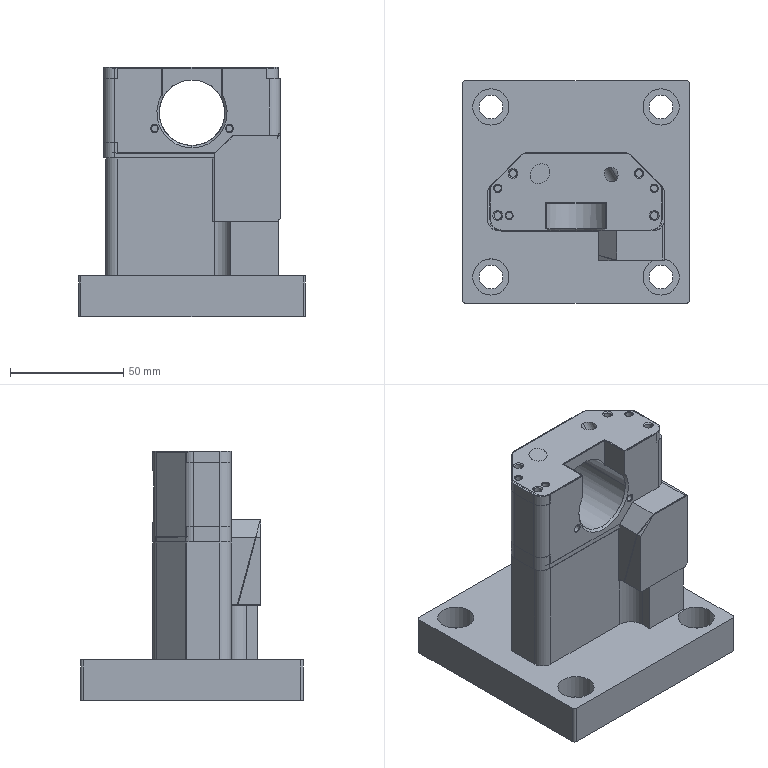NC program | NX | posted with a generic post | part box 100 x 98 x 110 mm
Lines 5823 to 6635 of 6635:
(3_AXIS_DEBURRING , TOOL : R1.75)
N11374 T07 M6
N11376 G54
N11378 G17 G0 G90 X41.123 Y0.273 B0. C0. S4500 M3
N11380 G43 Z67.959 H7
N11382 Z35.96
N11384 G94 G1 X41.109 Y0.272 Z35.792 F540.
N11386 X41.071 Y0.27 Z35.627
N11388 X41.011 Y0.267 Z35.466
N11390 X40.933 Y0.263 Z35.309
N11392 X40.736 Y0.251 Z35.017
N11394 X40.505 Y0.239 Z34.758
N11396 X40.415 Y0.21 Z34.668
N11398 X40.335 Y0.142 Z34.587
N11400 X40.264 Y0.042 Z34.517
N11402 X40.205 Y-0.082 Z34.457
N11404 X40.158 Y-0.222 Z34.41
N11406 X40.123 Y-0.371 Z34.375
N11408 X40.102 Y-0.519 Z34.353
N11410 X40.095 Y-0.66 Z34.346
N11412 X40.096 Y-1.682 F600.
N11414 Y-2.643
N11416 Y-3.603
N11418 Y-4.564
N11420 Y-5.525
N11422 Y-6.486
N11424 Y-7.446
N11426 Y-8.407
N11428 Y-9.368
N11430 Y-10.329
N11432 Y-11.289
N11434 Y-12.25
N11436 X40.104 Y-12.388 Z34.354
N11438 X40.126 Y-12.535 Z34.376
N11440 X40.161 Y-12.681 Z34.411
N11442 X40.209 Y-12.819 Z34.459
N11444 X40.269 Y-12.941 Z34.519
N11446 X40.339 Y-13.038 Z34.589
N11448 X40.42 Y-13.102 Z34.67
N11450 X40.508 Y-13.125 Z34.758
N11452 X40.74 Z35.017
N11454 X40.937 Z35.31
N11456 X41.015 Z35.466
N11458 X41.075 Z35.627
N11460 X41.114 Z35.793
N11462 X41.127 Z35.961
N11464 X41.164 Y-13.127 Z36.375
N11466 X41.206 Y-13.134 Z36.797
N11468 X41.254 Y-13.144 Z37.224
N11470 X41.306 Y-13.157 Z37.655
N11472 X41.36 Y-13.172 Z38.09
N11474 X41.416 Y-13.188 Z38.526
N11476 X41.473 Y-13.205 Z38.963
N11478 X41.528 Y-13.22 Z39.399
N11480 X41.582 Y-13.235 Z39.832
N11482 X41.632 Y-13.247 Z40.262
N11484 X41.678 Y-13.256 Z40.688
N11486 X41.719 Y-13.261 Z41.107
N11488 X41.753 Y-13.262 Z41.518
N11490 X41.78 Y-13.258 Z41.921
N11492 X41.797 Y-13.247 Z42.313
N11494 X41.805 Y-13.229 Z42.694
N11496 X41.801 Y-13.203 Z43.063
N11498 X41.784 Y-13.169 Z43.416
N11500 X41.754 Y-13.125 Z43.755
N11502 X41.704 Y-13.066 Z44.092
N11504 X41.629 Y-12.991 Z44.421
N11506 X41.531 Y-12.899 Z44.742
N11508 X41.411 Y-12.792 Z45.055
N11510 X41.268 Y-12.669 Z45.361
N11512 X41.104 Y-12.532 Z45.658
N11514 X40.919 Y-12.381 Z45.948
N11516 X40.714 Y-12.215 Z46.229
N11518 X40.49 Y-12.037 Z46.502
N11520 X40.247 Y-11.845 Z46.767
N11522 X39.986 Y-11.641 Z47.024
N11524 X39.707 Y-11.424 Z47.273
N11526 X39.412 Y-11.197 Z47.513
N11528 X39.101 Y-10.958 Z47.745
N11530 X38.774 Y-10.708 Z47.968
N11532 X38.433 Y-10.449 Z48.183
N11534 X38.077 Y-10.179 Z48.39
N11536 X37.708 Y-9.9 Z48.588
N11538 X37.327 Y-9.613 Z48.777
N11540 X36.933 Y-9.317 Z48.957
N11542 X36.528 Y-9.013 Z49.129
N11544 X36.112 Y-8.702 Z49.293
N11546 X35.686 Y-8.383 Z49.447
N11548 X35.251 Y-8.058 Z49.593
N11550 X34.807 Y-7.728 Z49.729
N11552 X34.355 Y-7.391 Z49.857
N11554 X33.895 Y-7.049 Z49.976
N11556 X33.429 Y-6.703 Z50.085
N11558 X32.956 Y-6.352 Z50.186
N11560 X32.478 Y-5.998 Z50.277
N11562 X31.996 Y-5.64 Z50.359
N11564 X31.509 Y-5.279 Z50.433
N11566 X31.019 Y-4.916 Z50.496
N11568 X30.526 Y-4.551 Z50.551
N11570 X30.031 Y-4.184 Z50.596
N11572 X29.535 Y-3.817 Z50.631
N11574 X29.038 Y-3.448 Z50.657
N11576 X28.541 Y-3.08 Z50.674
N11578 X28.044 Y-2.712 Z50.681
N11580 X27.549 Y-2.345 Z50.678
N11582 X27.055 Y-1.978 Z50.666
N11584 X26.564 Y-1.614 Z50.644
N11586 X26.076 Y-1.252 Z50.612
N11588 X25.592 Y-0.892 Z50.571
N11590 X25.113 Y-0.535 Z50.519
N11592 X24.639 Y-0.182 Z50.458
N11594 X24.171 Y0.167 Z50.387
N11596 X23.709 Y0.512 Z50.305
N11598 X23.255 Y0.851 Z50.214
N11600 X22.808 Y1.186 Z50.112
N11602 X22.37 Y1.515 Z50.001
N11604 X21.942 Y1.837 Z49.879
N11606 X21.523 Y2.153 Z49.747
N11608 X21.115 Y2.461 Z49.604
N11610 X20.717 Y2.762 Z49.452
N11612 X20.332 Y3.055 Z49.289
N11614 X19.959 Y3.339 Z49.115
N11616 X19.6 Y3.615 Z48.931
N11618 X19.254 Y3.881 Z48.736
N11620 X18.923 Y4.137 Z48.531
N11622 X18.607 Y4.382 Z48.315
N11624 X18.307 Y4.617 Z48.089
N11626 X18.024 Y4.841 Z47.851
N11628 X17.758 Y5.052 Z47.603
N11630 X17.509 Y5.252 Z47.345
N11632 X17.279 Y5.439 Z47.075
N11634 X17.069 Y5.613 Z46.794
N11636 X16.878 Y5.773 Z46.503
N11638 X16.708 Y5.919 Z46.2
N11640 X16.558 Y6.051 Z45.886
N11642 X16.431 Y6.168 Z45.561
N11644 X16.326 Y6.269 Z45.225
N11646 X16.245 Y6.355 Z44.878
N11648 X16.187 Y6.424 Z44.52
N11650 X16.154 Y6.476 Z44.15
N11652 X16.146 Y6.512 Z43.769
N11654 X16.149 Y6.521 Z43.623
N11656 X16.154 Y6.528 Z43.474
N11658 X16.162 Y6.534 Z43.323
N11660 X16.171 Y6.539 Z43.17
N11662 X16.182 Y6.543 Z43.016
N11664 X16.195 Y6.545 Z42.859
N11666 X16.209 Y6.547 Z42.701
N11668 X16.224 Y6.548 Z42.541
N11670 X16.24 Z42.381
N11672 X16.256 Z42.219
N11674 X16.274 Z42.058
N11676 X16.291 Y6.547 Z41.895
N11678 X16.309 Y6.546 Z41.733
N11680 X16.326 Y6.545 Z41.57
N11682 X16.344 Z41.408
N11684 X16.361 Y6.544 Z41.247
N11686 X16.377 Z41.086
N11688 X16.392 Y6.545 Z40.926
N11690 X16.406 Y6.547 Z40.768
N11692 X16.421 Y6.548 Z40.602 F540.
N11694 X16.462 Y6.554 Z40.439
N11696 X16.525 Y6.562 Z40.281
N11698 X16.607 Y6.573 Z40.129
N11700 X16.706 Y6.586 Z39.985
N11702 X16.815 Y6.601 Z39.848
N11704 X17.056 Y6.633 Z39.605
N11706 X17.147 Y6.669 Z39.523
N11708 X17.225 Y6.744 Z39.453
N11710 X17.289 Y6.851 Z39.393
N11712 X17.34 Y6.98 Z39.345
N11714 X17.377 Y7.124 Z39.309
N11716 X17.401 Y7.274 Z39.285
N11718 X17.41 Y7.422 Z39.273
N11720 X17.404 Y7.56 Z39.275
N11722 X17.395 Y7.661 Z39.282 F600.
N11724 X17.384 Y7.766 Z39.288
N11726 X17.35 Y7.904 Z39.303
N11728 X17.316 Y8.043 Z39.317
N11730 X17.281 Y8.181 Z39.332
N11732 X17.247 Y8.32 Z39.346
N11734 X17.19 Y8.444 Z39.359
N11736 X17.133 Y8.567 Z39.372
N11738 X17.076 Y8.691 Z39.385
N11740 X16.985 Y8.824 Z39.4
N11742 X16.894 Y8.957 Z39.414
N11744 X16.804 Y9.09 Z39.429
N11746 X16.674 Y9.213 Z39.442
N11748 X16.545 Y9.336 Z39.454
N11750 X16.415 Y9.459 Z39.467
N11752 X16.279 Y9.556 Z39.482
N11754 X16.142 Y9.654 Z39.498
N11756 X16.002 Y9.715 Z39.506
N11758 X15.861 Y9.777 Z39.515
N11760 X15.721 Y9.838 Z39.523
N11762 X15.555 Y9.867 Z39.529
N11764 X15.388 Y9.895 Z39.535
N11766 X15.222 Y9.924 Z39.541
N11768 X15.062 Y9.923 Z39.548
N11770 X14.902 Y9.922 Z39.556
N11772 X14.753 Y9.893 Z39.563
N11774 X14.605 Y9.864 Z39.571
N11776 X14.456 Y9.835 Z39.578
N11778 X14.323 Y9.767 Z39.581
N11780 X14.19 Y9.699 Z39.584
N11782 X14.057 Y9.63 Z39.586
N11784 X13.942 Y9.513 Z39.582
N11786 X13.827 Y9.395 Z39.577
N11788 X13.713 Y9.277 Z39.572
N11790 X13.641 Y9.154 Z39.567
N11792 X13.569 Y9.031 Z39.561
N11794 X13.497 Y8.907 Z39.556
N11796 X13.448 Y8.755 Z39.545
N11798 X13.399 Y8.602 Z39.535
N11800 X13.375 Y8.425 Z39.525
N11802 X13.35 Y8.249 Z39.516
N11804 X13.326 Y8.072 Z39.507
N11806 X13.337 Y7.925 Z39.498
N11808 X13.348 Y7.777 Z39.489
N11810 X13.359 Y7.63 Z39.481
N11812 X13.397 Y7.461 Z39.472
N11814 X13.434 Y7.293 Z39.463
N11816 X13.518 Y7.111 Z39.447
N11818 X13.602 Y6.93 Z39.432
N11820 X13.686 Y6.748 Z39.416
N11822 X13.778 Y6.644 Z39.391
N11824 X13.87 Y6.539 Z39.366
N11826 X13.962 Y6.435 Z39.341
N11828 X14.066 Y6.32 Z39.335
N11830 X14.171 Y6.206 Z39.328
N11832 X14.276 Y6.091 Z39.322
N11834 X14.412 Y5.994 Z39.312
N11836 X14.549 Y5.897 Z39.302
N11838 X14.685 Y5.8 Z39.292
N11840 X14.784 Y5.773 Z39.264
N11842 X14.883 Y5.745 Z39.236
N11844 X14.982 Y5.717 Z39.209
N11846 X15.076 Y5.688 Z39.204
N11848 X15.17 Y5.659 Z39.2
N11850 X15.265 Y5.63 Z39.195
N11852 X15.359 Y5.601 Z39.191
N11854 X15.464 Y5.597 Z39.178
N11856 X15.568 Y5.594 Z39.166
N11858 X15.673 Y5.59 Z39.153
N11860 X15.777 Y5.587 Z39.141
N11862 X15.86 Y5.601 Z39.13
N11864 X15.943 Y5.615 Z39.119
N11866 X16.027 Y5.629 Z39.108
N11868 X16.111 Y5.646 Z39.117
N11870 X16.196 Y5.663 Z39.126
N11872 X16.281 Y5.68 Z39.135
N11874 X16.366 Y5.697 Z39.144
N11876 X16.436 Y5.748 Z39.129
N11878 X16.506 Y5.798 Z39.113
N11880 X16.575 Y5.849 Z39.098
N11882 X16.645 Y5.899 Z39.082
N11884 X16.717 Y5.955 Z39.095
N11886 X16.788 Y6.01 Z39.108
N11888 X16.86 Y6.065 Z39.121
N11890 X16.931 Y6.121 Z39.133
N11892 X16.983 Y6.187 Z39.142
N11894 X17.034 Y6.254 Z39.15
N11896 X17.085 Y6.32 Z39.158
N11898 X17.137 Y6.386 Z39.167
N11900 X17.169 Y6.466 Z39.164
N11902 X17.201 Y6.546 Z39.161
N11904 X17.233 Y6.626 Z39.158
N11906 X17.264 Y6.734 Z39.167
N11908 X17.294 Y6.843 Z39.176
N11910 X17.324 Y6.951 Z39.186
N11912 X17.354 Y7.06 Z39.195
N11914 X17.374 Y7.19 Z39.219
N11916 X17.395 Y7.321 Z39.243
N11918 X17.415 Y7.451 Z39.268
N11920 X17.405 Y7.556 Z39.275
N11922 X17.404 Y7.56
N11924 X17.383 Y7.697 Z39.291
N11926 X17.346 Y7.84 Z39.321
N11928 X17.294 Y7.98 Z39.363
N11930 X17.231 Y8.11 Z39.417
N11932 X17.156 Y8.222 Z39.481
N11934 X17.073 Y8.309 Z39.553
N11936 X16.982 Y8.361 Z39.633
N11938 X16.886 Y8.371 Z39.718
N11940 X16.645 Y8.339 Z39.961
N11942 X16.535 Y8.324 Z40.098
N11944 X16.437 Y8.311 Z40.243
N11946 X16.354 Y8.3 Z40.395
N11948 X16.291 Y8.292 Z40.553
N11950 X16.25 Y8.286 Z40.715
N11952 X16.236 Y8.284 Z40.881
N11954 G0 Z45.881
N11956 G1 X16.232 Z46.073
N11958 X16.221 Z46.263
N11960 X16.202 Z46.451
N11962 X16.176 Y8.283 Z46.636
N11964 X16.142 Z46.818
N11966 X16.102 Y8.282 Z46.999
N11968 X16.054 Y8.281 Z47.176
N11970 X16. Y8.28 Z47.352
N11972 X15.939 Y8.278 Z47.525
N11974 X15.871 Y8.277 Z47.695
N11976 X15.796 Y8.276 Z47.863
N11978 X15.715 Y8.274 Z48.029
N11980 X15.627 Y8.272 Z48.192
N11982 X15.533 Y8.27 Z48.353
N11984 X15.433 Y8.268 Z48.511
N11986 X15.327 Y8.266 Z48.667
N11988 X15.214 Y8.264 Z48.82
N11990 X15.096 Y8.261 Z48.971
N11992 X14.972 Y8.259 Z49.12
N11994 X14.842 Y8.256 Z49.266
N11996 X14.707 Y8.254 Z49.409
N11998 X14.566 Y8.251 Z49.55
N12000 X14.42 Y8.248 Z49.689
N12002 X14.268 Y8.245 Z49.825
N12004 X14.111 Y8.242 Z49.959
N12006 X13.949 Y8.238 Z50.09
N12008 X13.782 Y8.235 Z50.219
N12010 X13.61 Y8.231 Z50.346
N12012 X13.433 Y8.228 Z50.47
N12014 X13.251 Y8.224 Z50.591
N12016 X13.065 Y8.22 Z50.71
N12018 X12.874 Y8.217 Z50.826
N12020 X12.679 Y8.213 Z50.941
N12022 X12.48 Y8.209 Z51.052
N12024 X12.276 Y8.204 Z51.161
N12026 X12.068 Y8.2 Z51.268
N12028 X11.856 Y8.196 Z51.372
N12030 X11.641 Y8.192 Z51.474
N12032 X11.421 Y8.187 Z51.573
N12034 X11.198 Y8.183 Z51.669
N12036 X10.971 Y8.178 Z51.764
N12038 X10.741 Y8.173 Z51.855
N12040 X10.507 Y8.169 Z51.944
N12042 X10.27 Y8.164 Z52.031
N12044 X10.029 Y8.159 Z52.115
N12046 X9.786 Y8.154 Z52.197
N12048 X9.539 Y8.149 Z52.276
N12050 X9.29 Y8.144 Z52.353
N12052 X9.038 Y8.139 Z52.427
N12054 X8.783 Y8.134 Z52.499
N12056 X8.525 Y8.129 Z52.568
N12058 X8.265 Y8.123 Z52.635
N12060 X8.003 Y8.118 Z52.699
N12062 X7.738 Y8.113 Z52.761
N12064 X7.471 Y8.107 Z52.82
N12066 X7.202 Y8.102 Z52.877
N12068 X6.931 Y8.096 Z52.931
N12070 X6.658 Y8.091 Z52.983
N12072 X6.383 Y8.085 Z53.032
N12074 X6.106 Y8.08 Z53.078
N12076 X5.828 Y8.074 Z53.122
N12078 X5.549 Y8.068 Z53.164
N12080 X5.268 Y8.063 Z53.203
N12082 X4.985 Y8.057 Z53.24
N12084 X4.702 Y8.051 Z53.274
N12086 X4.417 Y8.046 Z53.305
N12088 X4.131 Y8.04 Z53.334
N12090 X3.845 Y8.034 Z53.361
N12092 X3.557 Y8.028 Z53.384
N12094 X3.269 Y8.022 Z53.406
N12096 X2.981 Y8.017 Z53.425
N12098 X2.691 Y8.011 Z53.441
N12100 X2.402 Y8.005 Z53.455
N12102 X2.112 Y7.999 Z53.466
N12104 X1.822 Y7.993 Z53.474
N12106 X1.532 Y7.987 Z53.481
N12108 X1.241 Y7.981 Z53.484
N12110 X0.951 Y7.976 Z53.485
N12112 X0.661 Y7.97 Z53.484
N12114 X0.372 Y7.964 Z53.479
N12116 X0.083 Y7.958 Z53.473
N12118 X-0.206 Y7.952 Z53.464
N12120 X-0.494 Y7.946 Z53.452
N12122 X-0.782 Y7.94 Z53.438
N12124 X-1.068 Y7.935 Z53.421
N12126 X-1.354 Y7.929 Z53.401
N12128 X-1.639 Y7.923 Z53.379
N12130 X-1.922 Y7.917 Z53.355
N12132 X-2.204 Y7.912 Z53.328
N12134 X-2.486 Y7.906 Z53.298
N12136 X-2.765 Y7.9 Z53.266
N12138 X-3.043 Y7.895 Z53.231
N12140 X-3.32 Y7.889 Z53.193
N12142 X-3.595 Y7.884 Z53.153
N12144 X-3.868 Y7.878 Z53.111
N12146 X-4.139 Y7.873 Z53.066
N12148 X-4.408 Y7.867 Z53.018
N12150 X-4.675 Y7.862 Z52.968
N12152 X-4.94 Y7.856 Z52.915
N12154 X-5.202 Y7.851 Z52.859
N12156 X-5.462 Y7.846 Z52.801
N12158 X-5.72 Y7.841 Z52.741
N12160 X-5.975 Y7.836 Z52.677
N12162 X-6.227 Y7.83 Z52.612
N12164 X-6.476 Y7.825 Z52.543
N12166 X-6.723 Y7.82 Z52.472
N12168 X-6.966 Y7.815 Z52.398
N12170 X-7.207 Y7.811 Z52.322
N12172 X-7.444 Y7.806 Z52.243
N12174 X-7.677 Y7.801 Z52.162
N12176 X-7.908 Y7.796 Z52.078
N12178 X-8.135 Y7.792 Z51.991
N12180 X-8.358 Y7.787 Z51.902
N12182 X-8.578 Y7.783 Z51.81
N12184 X-8.793 Y7.779 Z51.716
N12186 X-9.005 Y7.774 Z51.619
N12188 X-9.213 Y7.77 Z51.519
N12190 X-9.417 Y7.766 Z51.417
N12192 X-9.616 Y7.762 Z51.312
N12194 X-9.811 Y7.758 Z51.204
N12196 X-10.002 Y7.754 Z51.094
N12198 X-10.188 Y7.75 Z50.981
N12200 X-10.37 Y7.747 Z50.866
N12202 X-10.547 Y7.743 Z50.748
N12204 X-10.719 Y7.74 Z50.627
N12206 X-10.886 Y7.736 Z50.504
N12208 X-11.048 Y7.733 Z50.378
N12210 X-11.205 Y7.73 Z50.25
N12212 X-11.356 Y7.727 Z50.119
N12214 X-11.503 Y7.724 Z49.985
N12216 X-11.644 Y7.721 Z49.848
N12218 X-11.779 Y7.718 Z49.709
N12220 X-11.909 Y7.716 Z49.567
N12222 X-12.033 Y7.713 Z49.423
N12224 X-12.151 Y7.711 Z49.276
N12226 X-12.264 Y7.708 Z49.126
N12228 X-12.37 Y7.706 Z48.974
N12230 X-12.47 Y7.704 Z48.819
N12232 X-12.564 Y7.702 Z48.662
N12234 X-12.652 Y7.701 Z48.501
N12236 X-12.733 Y7.699 Z48.338
N12238 X-12.808 Y7.697 Z48.173
N12240 X-12.876 Y7.696 Z48.005
N12242 X-12.937 Y7.695 Z47.834
N12244 X-12.991 Y7.694 Z47.66
N12246 X-13.039 Y7.693 Z47.484
N12248 X-13.079 Y7.692 Z47.305
N12250 X-13.113 Y7.691 Z47.124
N12252 X-13.139 Z46.939
N12254 X-13.158 Y7.69 Z46.753
N12256 X-13.169 Z46.563
N12258 X-13.173 Z46.371
N12260 G0 Z41.37
N12262 G1 X-13.163 Z41.195 F540.
N12264 X-13.135 Y7.689 Z41.022
N12266 X-13.034 Y7.688 Z40.681
N12268 X-12.886 Y7.685 Z40.354
N12270 X-12.709 Y7.682 Z40.045
N12272 X-12.642 Y7.705 Z39.939
N12274 X-12.581 Y7.768 Z39.844
N12276 X-12.526 Y7.864 Z39.761
N12278 X-12.478 Y7.985 Z39.692
N12280 X-12.439 Y8.123 Z39.636
N12282 X-12.409 Y8.269 Z39.595
N12284 X-12.39 Y8.414 Z39.571
N12286 X-12.381 Y8.552 Z39.564
N12288 X-12.379 Y8.626 Z39.565 F600.
N12290 X-12.375 Y8.839 Z39.568
N12292 X-12.377 Y9.048 Z39.582
N12294 X-12.378 Y9.257 Z39.596
N12296 X-12.431 Y9.451 Z39.594
N12298 X-12.483 Y9.644 Z39.592
N12300 X-12.556 Y9.863 Z39.599
N12302 X-12.63 Y10.081 Z39.607
N12304 X-12.692 Y10.227 Z39.617
N12306 X-12.754 Y10.373 Z39.626
N12308 X-12.877 Y10.516 Z39.62
N12310 X-12.999 Y10.66 Z39.613
N12312 X-13.184 Y10.849 Z39.619
N12314 X-13.368 Y11.038 Z39.624
N12316 X-13.621 Y11.186 Z39.622
N12318 X-13.874 Y11.334 Z39.619
N12320 X-14.054 Y11.392 Z39.614
N12322 X-14.235 Y11.45 Z39.608
N12324 X-14.481 Y11.526 Z39.614
N12326 X-14.747 Y11.538 Z39.603
N12328 X-15.013 Y11.55 Z39.591
N12330 X-15.215 Y11.543 Z39.59
N12332 X-15.417 Y11.537 Z39.589
N12334 X-15.622 Y11.482 Z39.575
N12336 X-15.826 Y11.427 Z39.56
N12338 X-16.033 Y11.364 Z39.555
N12340 X-16.239 Y11.302 Z39.55
N12342 X-16.433 Y11.2 Z39.534
N12344 X-16.626 Y11.098 Z39.517
N12346 X-16.868 Y10.957 Z39.509
N12348 X-17.11 Y10.817 Z39.502
N12350 X-17.24 Y10.698 Z39.482
N12352 X-17.369 Y10.579 Z39.462
N12354 X-17.533 Y10.409 Z39.439
N12356 X-17.698 Y10.24 Z39.416
N12358 X-17.861 Y10.076
N12360 X-18.024 Y9.913
N12362 X-18.139 Y9.73 Z39.39
N12364 X-18.254 Y9.548 Z39.364
N12366 X-18.432 Y9.207 Z39.333
N12368 X-18.61 Y8.865 Z39.301
N12370 X-18.668 Y8.678 Z39.277
N12372 X-18.727 Y8.49 Z39.253
N12374 X-18.785 Y8.302 Z39.229
N12376 X-18.835 Y8.069 Z39.218
N12378 X-18.886 Y7.837 Z39.207
N12380 X-18.936 Y7.604 Z39.196
N12382 X-18.949 Y7.483 Z39.197
N12384 X-18.963 Y7.362 Z39.198
N12386 X-18.976 Y7.241 Z39.199
N12388 X-18.961 Y7.128 Z39.178
N12390 X-18.946 Y7.016 Z39.157
N12392 X-18.931 Y6.903 Z39.136
N12394 X-18.91 Y6.707 Z39.139
N12396 X-18.889 Y6.511 Z39.141
N12398 X-18.846 Y6.408 Z39.115
N12400 X-18.802 Y6.305 Z39.088
N12402 X-18.759 Y6.202 Z39.062
N12404 X-18.718 Y6.082 Z39.073
N12406 X-18.678 Y5.963 Z39.084
N12408 X-18.637 Y5.843 Z39.095
N12410 X-18.582 Y5.779 Z39.068
N12412 X-18.527 Y5.715 Z39.041
N12414 X-18.471 Y5.652 Z39.014
N12416 X-18.422 Y5.567 Z39.033
N12418 X-18.373 Y5.482 Z39.053
N12420 X-18.324 Y5.397 Z39.072
N12422 X-18.247 Y5.33 Z39.065
N12424 X-18.169 Y5.263 Z39.057
N12426 X-18.092 Y5.196 Z39.05
N12428 X-18.015 Y5.129 Z39.043
N12430 X-17.916 Y5.075 Z39.033
N12432 X-17.817 Y5.022 Z39.023
N12434 X-17.718 Y4.968 Z39.013
N12436 X-17.619 Y4.914 Z39.003
N12438 X-17.532 Y4.863 Z39.032
N12440 X-17.446 Y4.812 Z39.06
N12442 X-17.36 Y4.761 Z39.088
N12444 X-17.259 Y4.747 Z39.069
N12446 X-17.158 Y4.733 Z39.049
N12448 X-17.013 Y4.71 Z39.058
N12450 X-16.868 Y4.687 Z39.067
N12452 X-16.723 Y4.664 Z39.076
N12454 X-16.609 Y4.649 Z39.101
N12456 X-16.496 Y4.635 Z39.127
N12458 X-16.383 Y4.621 Z39.153
N12460 X-16.202 Y4.651 Z39.147
N12462 X-16.022 Y4.682 Z39.142
N12464 X-15.893 Y4.698 Z39.165
N12466 X-15.764 Y4.714 Z39.189
N12468 X-15.635 Y4.73 Z39.213
N12470 X-15.454 Y4.806 Z39.206
N12472 X-15.273 Y4.882 Z39.2
N12474 X-15.032 Y4.992 Z39.221
N12476 X-14.791 Y5.102 Z39.242
N12478 X-14.653 Y5.185 Z39.251
N12480 X-14.516 Y5.269 Z39.26
N12482 X-14.33 Y5.399 Z39.279
N12484 X-14.143 Y5.53 Z39.297
N12486 X-13.959 Y5.666 Z39.333
N12488 X-13.774 Y5.802 Z39.368
N12490 X-13.626 Y5.957 Z39.381
N12492 X-13.478 Y6.113 Z39.395
N12494 X-13.258 Y6.433 Z39.41
N12496 X-13.037 Y6.754 Z39.425
N12498 X-12.933 Y6.934 Z39.444
N12500 X-12.83 Y7.114 Z39.463
N12502 X-12.727 Y7.294 Z39.482
N12504 X-12.603 Y7.651 Z39.505
N12506 X-12.479 Y8.009 Z39.528
N12508 X-12.431 Y8.211 Z39.545
N12510 X-12.384 Y8.413 Z39.562
N12512 X-12.381 Y8.552 Z39.564
N12514 X-12.384 Y8.691 Z39.575
N12516 X-12.397 Y8.838 Z39.603
N12518 X-12.42 Y8.984 Z39.648
N12520 X-12.453 Y9.123 Z39.708
N12522 X-12.495 Y9.245 Z39.781
N12524 X-12.546 Y9.343 Z39.867
N12526 X-12.605 Y9.408 Z39.964
N12528 X-12.671 Y9.432 Z40.072
N12530 X-12.848 Y9.435 Z40.381
N12532 X-12.996 Y9.437 Z40.708
N12534 X-13.097 Y9.439 Z41.048
N12536 X-13.125 Z41.222
N12538 X-13.135 Z41.397
N12540 G0 Z46.397
N12542 G1 X-13.138 Y9.436 Z46.635
N12544 X-13.149 Y9.428 Z46.867
N12546 X-13.167 Y9.413 Z47.095
N12548 X-13.192 Y9.393 Z47.318
N12550 X-13.224 Y9.368 Z47.537
N12552 X-13.262 Y9.337 Z47.752
N12554 X-13.307 Y9.3 Z47.962
N12556 X-13.359 Y9.258 Z48.167
N12558 X-13.418 Y9.211 Z48.368
N12560 X-13.482 Y9.159 Z48.565
N12562 X-13.553 Y9.102 Z48.757
N12564 X-13.631 Y9.04 Z48.945
N12566 X-13.714 Y8.972 Z49.129
N12568 X-13.803 Y8.9 Z49.309
N12570 X-13.899 Y8.824 Z49.484
N12572 X-14. Y8.742 Z49.654
N12574 X-14.107 Y8.656 Z49.821
N12576 X-14.219 Y8.565 Z49.983
N12578 X-14.338 Y8.47 Z50.141
N12580 X-14.461 Y8.37 Z50.295
N12582 X-14.59 Y8.266 Z50.445
N12584 X-14.724 Y8.158 Z50.59
N12586 X-14.864 Y8.046 Z50.732
N12588 X-15.008 Y7.929 Z50.869
N12590 X-15.157 Y7.809 Z51.002
N12592 X-15.312 Y7.685 Z51.131
N12594 X-15.471 Y7.556 Z51.256
N12596 X-15.634 Y7.424 Z51.377
N12598 X-15.803 Y7.289 Z51.494
N12600 X-15.976 Y7.149 Z51.606
N12602 X-16.153 Y7.007 Z51.715
N12604 X-16.334 Y6.86 Z51.82
N12606 X-16.52 Y6.71 Z51.921
N12608 X-16.71 Y6.557 Z52.018
N12610 X-16.904 Y6.401 Z52.111
N12612 X-17.102 Y6.242 Z52.2
N12614 X-17.303 Y6.079 Z52.285
N12616 X-17.509 Y5.914 Z52.366
N12618 X-17.718 Y5.745 Z52.444
N12620 X-17.93 Y5.574 Z52.517
N12622 X-18.146 Y5.4 Z52.587
N12624 X-18.365 Y5.223 Z52.653
N12626 X-18.588 Y5.044 Z52.715
N12628 X-18.814 Y4.862 Z52.774
N12630 X-19.042 Y4.677 Z52.829
N12632 X-19.274 Y4.49 Z52.88
N12634 X-19.509 Y4.301 Z52.927
N12636 X-19.746 Y4.11 Z52.97
N12638 X-19.986 Y3.916 Z53.01
N12640 X-20.229 Y3.721 Z53.047
N12642 X-20.474 Y3.523 Z53.079
N12644 X-20.722 Y3.324 Z53.108
N12646 X-20.971 Y3.122 Z53.134
N12648 X-21.223 Y2.919 Z53.156
N12650 X-21.478 Y2.714 Z53.174
N12652 X-21.734 Y2.508 Z53.189
N12654 X-21.992 Y2.3 Z53.2
N12656 X-22.252 Y2.09 Z53.208
N12658 X-22.513 Y1.88 Z53.212
N12660 X-22.776 Y1.667 Z53.213
N12662 X-23.041 Y1.454 Z53.21
N12664 X-23.307 Y1.239 Z53.204
N12666 X-23.575 Y1.024 Z53.195
N12668 X-23.844 Y0.807 Z53.182
N12670 X-24.114 Y0.59 Z53.166
N12672 X-24.385 Y0.371 Z53.146
N12674 X-24.656 Y0.152 Z53.123
N12676 X-24.929 Y-0.068 Z53.097
N12678 X-25.203 Y-0.289 Z53.067
N12680 X-25.477 Y-0.51 Z53.035
N12682 X-25.752 Y-0.731 Z52.999
N12684 X-26.027 Y-0.953 Z52.959
N12686 X-26.303 Y-1.175 Z52.917
N12688 X-26.579 Y-1.398 Z52.871
N12690 X-26.855 Y-1.62 Z52.822
N12692 X-27.131 Y-1.843 Z52.77
N12694 X-27.407 Y-2.065 Z52.715
N12696 X-27.683 Y-2.288 Z52.657
N12698 X-27.959 Y-2.51 Z52.595
N12700 X-28.235 Y-2.733 Z52.531
N12702 X-28.51 Y-2.955 Z52.463
N12704 X-28.785 Y-3.176 Z52.392
N12706 X-29.059 Y-3.397 Z52.318
N12708 X-29.333 Y-3.618 Z52.242
N12710 X-29.606 Y-3.838 Z52.162
N12712 X-29.877 Y-4.057 Z52.079
N12714 X-30.148 Y-4.275 Z51.994
N12716 X-30.418 Y-4.493 Z51.905
N12718 X-30.687 Y-4.709 Z51.813
N12720 X-30.955 Y-4.925 Z51.719
N12722 X-31.221 Y-5.14 Z51.622
N12724 X-31.486 Y-5.353 Z51.521
N12726 X-31.749 Y-5.565 Z51.418
N12728 X-32.01 Y-5.776 Z51.313
N12730 X-32.27 Y-5.985 Z51.204
N12732 X-32.528 Y-6.193 Z51.092
N12734 X-32.784 Y-6.4 Z50.978
N12736 X-33.039 Y-6.605 Z50.861
N12738 X-33.291 Y-6.808 Z50.741
N12740 X-33.54 Y-7.009 Z50.619
N12742 X-33.788 Y-7.209 Z50.494
N12744 X-34.033 Y-7.406 Z50.366
N12746 X-34.276 Y-7.602 Z50.235
N12748 X-34.516 Y-7.796 Z50.102
N12750 X-34.753 Y-7.987 Z49.966
N12752 X-34.988 Y-8.176 Z49.828
N12754 X-35.22 Y-8.363 Z49.687
N12756 X-35.448 Y-8.547 Z49.543
N12758 X-35.674 Y-8.729 Z49.397
N12760 X-35.897 Y-8.909 Z49.248
N12762 X-36.116 Y-9.085 Z49.097
N12764 X-36.332 Y-9.26 Z48.943
N12766 X-36.544 Y-9.431 Z48.787
N12768 X-36.753 Y-9.599 Z48.629
N12770 X-36.959 Y-9.765 Z48.468
N12772 X-37.16 Y-9.927 Z48.304
N12774 X-37.358 Y-10.087 Z48.138
N12776 X-37.552 Y-10.243 Z47.97
N12778 X-37.742 Y-10.396 Z47.799
N12780 X-37.928 Y-10.546 Z47.626
N12782 X-38.109 Y-10.692 Z47.451
N12784 X-38.286 Y-10.835 Z47.273
N12786 X-38.459 Y-10.974 Z47.093
N12788 X-38.628 Y-11.11 Z46.911
N12790 X-38.791 Y-11.242 Z46.727
N12792 X-38.95 Y-11.37 Z46.54
N12794 X-39.105 Y-11.495 Z46.351
N12796 X-39.254 Y-11.615 Z46.16
N12798 X-39.398 Y-11.731 Z45.967
N12800 X-39.538 Y-11.844 Z45.771
N12802 X-39.672 Y-11.952 Z45.573
N12804 X-39.801 Y-12.056 Z45.374
N12806 X-39.924 Y-12.155 Z45.172
N12808 X-40.043 Y-12.251 Z44.968
N12810 X-40.155 Y-12.341 Z44.762
N12812 X-40.262 Y-12.428 Z44.554
N12814 X-40.363 Y-12.509 Z44.344
N12816 X-40.459 Y-12.586 Z44.132
N12818 X-40.548 Y-12.658 Z43.918
N12820 X-40.631 Y-12.725 Z43.701
N12822 X-40.709 Y-12.788 Z43.483
N12824 X-40.78 Y-12.845 Z43.263
N12826 X-40.844 Y-12.897 Z43.042
N12828 X-40.903 Y-12.944 Z42.818
N12830 X-40.955 Y-12.986 Z42.592
N12832 X-41. Y-13.022 Z42.365
N12834 X-41.038 Y-13.053 Z42.135
N12836 X-41.07 Y-13.079 Z41.904
N12838 X-41.095 Y-13.099 Z41.671
N12840 X-41.113 Y-13.113 Z41.436
N12842 X-41.124 Y-13.122 Z41.199
N12844 X-41.127 Y-13.125 Z40.961
N12846 G0 Z35.961
N12848 G1 X-41.114 Z35.793 F540.
N12850 X-41.075 Z35.627
N12852 X-41.015 Z35.466
N12854 X-40.937 Z35.31
N12856 X-40.74 Z35.017
N12858 X-40.508 Z34.758
N12860 X-40.42 Y-13.102 Z34.67
N12862 X-40.339 Y-13.038 Z34.589
N12864 X-40.269 Y-12.941 Z34.519
N12866 X-40.209 Y-12.819 Z34.459
N12868 X-40.161 Y-12.681 Z34.411
N12870 X-40.126 Y-12.535 Z34.376
N12872 X-40.104 Y-12.388 Z34.354
N12874 X-40.096 Y-12.25 Z34.346
N12876 Y-11.289 F600.
N12878 Y-10.329
N12880 Y-9.368
N12882 Y-8.407
N12884 Y-7.446
N12886 Y-6.486
N12888 Y-5.525
N12890 Y-4.564
N12892 Y-3.603
N12894 Y-2.643
N12896 Y-1.682
N12898 X-40.095 Y-0.66
N12900 X-40.102 Y-0.519 Z34.353
N12902 X-40.123 Y-0.371 Z34.375
N12904 X-40.158 Y-0.222 Z34.41
N12906 X-40.205 Y-0.082 Z34.457
N12908 X-40.264 Y0.042 Z34.517
N12910 X-40.335 Y0.142 Z34.587
N12912 X-40.415 Y0.21 Z34.668
N12914 X-40.505 Y0.239 Z34.758
N12916 X-40.736 Y0.251 Z35.017
N12918 X-40.933 Y0.263 Z35.309
N12920 X-41.011 Y0.267 Z35.466
N12922 X-41.071 Y0.27 Z35.627
N12924 X-41.109 Y0.272 Z35.792
N12926 X-41.123 Y0.273 Z35.96
N12928 G0 Z67.959
N12930 M5
(PLANAR_MILL_23 , TOOL : 点孔D8-79-90度)
N12932 T15 M6
N12934 G54
N12936 G19 G0 G90 Y59. Z10.6 B-180. C-90. S4500 M3
N12938 G43 X-1.779 H15
N12940 Y40.5
N12942 G94 G1 Y38.5 F800.
N12944 X0.721
N12946 X12.25
N12948 X14.75
N12950 Y40.5
N12952 G0 Y59.
N12954 M5
(DRILLING_6 , TOOL : D29镗刀)
N12956 T16 M6
N12958 G54
N12960 G19 G0 G90 Y18.05 Z20. B-180. C0. S1200 M3
N12962 G43 X0. H16
N12964 G17 G94 G76 G99 Y-18.75 F60. R20.
N12966 G80
(DRILLING_6_COPY , TOOL : D29镗刀)
N12968 G19 G76 X0. Y-18.75 Z20. F60. R0.
N12970 G80
N12972 M5
N12974 M2